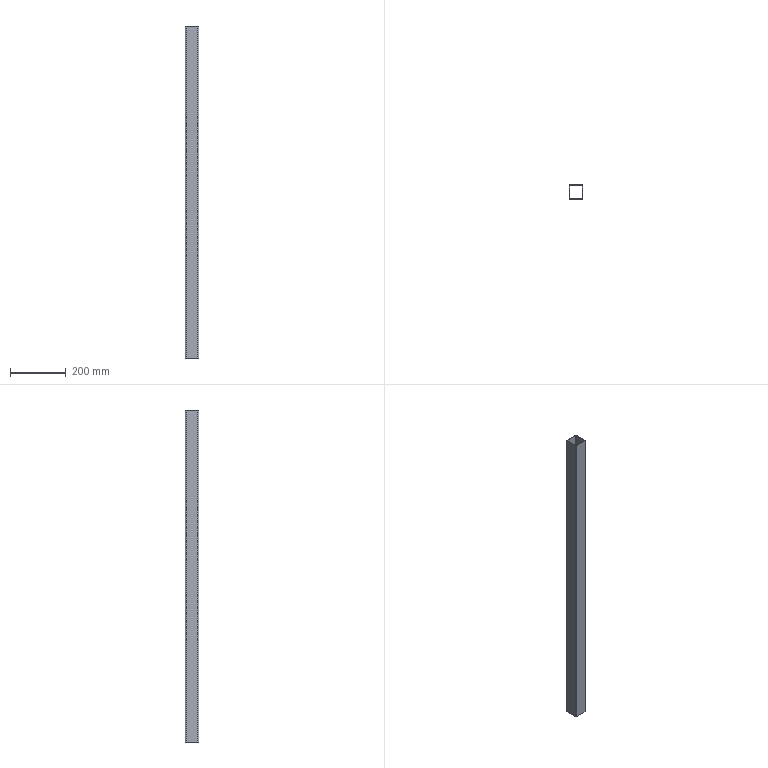Part | SolidWorks | features BaseBody 1 | 1 solid | 18 faces | box 50 x 50 x 1196 mm | volume 446944 mm3 | plane 10 | cylinder 8 | commonest cylinder face diameters 4 x4 8 x4
STEP:
#1=CARTESIAN_POINT('',(-23.,21.,-598.));
#2=VERTEX_POINT('',#1);
#3=CARTESIAN_POINT('',(-23.,-21.,-598.));
#4=VERTEX_POINT('',#3);
#5=CARTESIAN_POINT('',(-23.,21.,-598.));
#6=DIRECTION('',(0.,-1.,0.));
#7=VECTOR('',#6,1000.);
#8=LINE('',#5,#7);
#9=EDGE_CURVE('',#2,#4,#8,.T.);
#10=ORIENTED_EDGE('',*,*,#9,.F.);
#11=CARTESIAN_POINT('',(-23.,21.,598.));
#12=VERTEX_POINT('',#11);
#13=CARTESIAN_POINT('',(-23.,21.,598.));
#14=DIRECTION('',(0.,0.,-1.));
#15=VECTOR('',#14,1000.);
#16=LINE('',#13,#15);
#17=EDGE_CURVE('',#12,#2,#16,.T.);
#18=ORIENTED_EDGE('',*,*,#17,.F.);
#19=CARTESIAN_POINT('',(-23.,-21.,598.));
#20=VERTEX_POINT('',#19);
#21=CARTESIAN_POINT('',(-23.,21.,598.));
#22=DIRECTION('',(0.,-1.,0.));
#23=VECTOR('',#22,1000.);
#24=LINE('',#21,#23);
#25=EDGE_CURVE('',#12,#20,#24,.T.);
#26=ORIENTED_EDGE('',*,*,#25,.T.);
#27=CARTESIAN_POINT('',(-23.,-21.,598.));
#28=DIRECTION('',(0.,0.,-1.));
#29=VECTOR('',#28,1000.);
#30=LINE('',#27,#29);
#31=EDGE_CURVE('',#20,#4,#30,.T.);
#32=ORIENTED_EDGE('',*,*,#31,.T.);
#33=EDGE_LOOP('',(#10,#18,#26,#32));
#34=FACE_OUTER_BOUND('',#33,.T.);
#35=CARTESIAN_POINT('',(-23.,21.,598.));
#36=DIRECTION('',(1.,0.,0.));
#37=DIRECTION('',(0.,1.,0.));
#38=AXIS2_PLACEMENT_3D('',#35,#36,#37);
#39=PLANE('',#38);
#40=ADVANCED_FACE('',(#34),#39,.T.);
#41=CARTESIAN_POINT('',(-21.,23.,-598.));
#42=VERTEX_POINT('',#41);
#43=CARTESIAN_POINT('',(-21.,21.,-598.));
#44=DIRECTION('',(0.,0.,1.));
#45=DIRECTION('',(1.,0.,0.));
#46=AXIS2_PLACEMENT_3D('',#43,#44,#45);
#47=CIRCLE('',#46,2.);
#48=EDGE_CURVE('',#42,#2,#47,.T.);
#49=ORIENTED_EDGE('',*,*,#48,.F.);
#50=CARTESIAN_POINT('',(-21.,23.,598.));
#51=VERTEX_POINT('',#50);
#52=CARTESIAN_POINT('',(-21.,23.,598.));
#53=DIRECTION('',(0.,0.,-1.));
#54=VECTOR('',#53,1000.);
#55=LINE('',#52,#54);
#56=EDGE_CURVE('',#51,#42,#55,.T.);
#57=ORIENTED_EDGE('',*,*,#56,.F.);
#58=CARTESIAN_POINT('',(-21.,21.,598.));
#59=DIRECTION('',(0.,0.,1.));
#60=DIRECTION('',(1.,0.,0.));
#61=AXIS2_PLACEMENT_3D('',#58,#59,#60);
#62=CIRCLE('',#61,2.);
#63=EDGE_CURVE('',#51,#12,#62,.T.);
#64=ORIENTED_EDGE('',*,*,#63,.T.);
#65=ORIENTED_EDGE('',*,*,#17,.T.);
#66=EDGE_LOOP('',(#49,#57,#64,#65));
#67=FACE_OUTER_BOUND('',#66,.T.);
#68=CARTESIAN_POINT('',(-21.,21.,598.));
#69=DIRECTION('',(0.,0.,-1.));
#70=DIRECTION('',(-1.,0.,0.));
#71=AXIS2_PLACEMENT_3D('',#68,#69,#70);
#72=CYLINDRICAL_SURFACE('',#71,2.);
#73=ADVANCED_FACE('',(#67),#72,.F.);
#74=CARTESIAN_POINT('',(21.,23.,-598.));
#75=VERTEX_POINT('',#74);
#76=CARTESIAN_POINT('',(-21.,23.,-598.));
#77=DIRECTION('',(-1.,0.,0.));
#78=VECTOR('',#77,1000.);
#79=LINE('',#76,#78);
#80=EDGE_CURVE('',#75,#42,#79,.T.);
#81=ORIENTED_EDGE('',*,*,#80,.F.);
#82=CARTESIAN_POINT('',(21.,23.,598.));
#83=VERTEX_POINT('',#82);
#84=CARTESIAN_POINT('',(21.,23.,598.));
#85=DIRECTION('',(0.,0.,-1.));
#86=VECTOR('',#85,1000.);
#87=LINE('',#84,#86);
#88=EDGE_CURVE('',#83,#75,#87,.T.);
#89=ORIENTED_EDGE('',*,*,#88,.F.);
#90=CARTESIAN_POINT('',(-21.,23.,598.));
#91=DIRECTION('',(-1.,0.,0.));
#92=VECTOR('',#91,1000.);
#93=LINE('',#90,#92);
#94=EDGE_CURVE('',#83,#51,#93,.T.);
#95=ORIENTED_EDGE('',*,*,#94,.T.);
#96=ORIENTED_EDGE('',*,*,#56,.T.);
#97=EDGE_LOOP('',(#81,#89,#95,#96));
#98=FACE_OUTER_BOUND('',#97,.T.);
#99=CARTESIAN_POINT('',(-21.,23.,598.));
#100=DIRECTION('',(0.,-1.,0.));
#101=DIRECTION('',(0.,0.,-1.));
#102=AXIS2_PLACEMENT_3D('',#99,#100,#101);
#103=PLANE('',#102);
#104=ADVANCED_FACE('',(#98),#103,.T.);
#105=CARTESIAN_POINT('',(23.,21.,-598.));
#106=VERTEX_POINT('',#105);
#107=CARTESIAN_POINT('',(21.,21.,-598.));
#108=DIRECTION('',(0.,0.,1.));
#109=DIRECTION('',(1.,0.,0.));
#110=AXIS2_PLACEMENT_3D('',#107,#108,#109);
#111=CIRCLE('',#110,2.);
#112=EDGE_CURVE('',#106,#75,#111,.T.);
#113=ORIENTED_EDGE('',*,*,#112,.F.);
#114=CARTESIAN_POINT('',(23.,21.,598.));
#115=VERTEX_POINT('',#114);
#116=CARTESIAN_POINT('',(23.,21.,598.));
#117=DIRECTION('',(0.,0.,-1.));
#118=VECTOR('',#117,1000.);
#119=LINE('',#116,#118);
#120=EDGE_CURVE('',#115,#106,#119,.T.);
#121=ORIENTED_EDGE('',*,*,#120,.F.);
#122=CARTESIAN_POINT('',(21.,21.,598.));
#123=DIRECTION('',(0.,0.,1.));
#124=DIRECTION('',(1.,0.,0.));
#125=AXIS2_PLACEMENT_3D('',#122,#123,#124);
#126=CIRCLE('',#125,2.);
#127=EDGE_CURVE('',#115,#83,#126,.T.);
#128=ORIENTED_EDGE('',*,*,#127,.T.);
#129=ORIENTED_EDGE('',*,*,#88,.T.);
#130=EDGE_LOOP('',(#113,#121,#128,#129));
#131=FACE_OUTER_BOUND('',#130,.T.);
#132=CARTESIAN_POINT('',(21.,21.,598.));
#133=DIRECTION('',(0.,0.,-1.));
#134=DIRECTION('',(-1.,0.,0.));
#135=AXIS2_PLACEMENT_3D('',#132,#133,#134);
#136=CYLINDRICAL_SURFACE('',#135,2.);
#137=ADVANCED_FACE('',(#131),#136,.F.);
#138=CARTESIAN_POINT('',(23.,-21.,-598.));
#139=VERTEX_POINT('',#138);
#140=CARTESIAN_POINT('',(23.,21.,-598.));
#141=DIRECTION('',(0.,1.,0.));
#142=VECTOR('',#141,1000.);
#143=LINE('',#140,#142);
#144=EDGE_CURVE('',#139,#106,#143,.T.);
#145=ORIENTED_EDGE('',*,*,#144,.F.);
#146=CARTESIAN_POINT('',(23.,-21.,598.));
#147=VERTEX_POINT('',#146);
#148=CARTESIAN_POINT('',(23.,-21.,598.));
#149=DIRECTION('',(0.,0.,-1.));
#150=VECTOR('',#149,1000.);
#151=LINE('',#148,#150);
#152=EDGE_CURVE('',#147,#139,#151,.T.);
#153=ORIENTED_EDGE('',*,*,#152,.F.);
#154=CARTESIAN_POINT('',(23.,21.,598.));
#155=DIRECTION('',(0.,1.,0.));
#156=VECTOR('',#155,1000.);
#157=LINE('',#154,#156);
#158=EDGE_CURVE('',#147,#115,#157,.T.);
#159=ORIENTED_EDGE('',*,*,#158,.T.);
#160=ORIENTED_EDGE('',*,*,#120,.T.);
#161=EDGE_LOOP('',(#145,#153,#159,#160));
#162=FACE_OUTER_BOUND('',#161,.T.);
#163=CARTESIAN_POINT('',(23.,21.,598.));
#164=DIRECTION('',(-1.,0.,0.));
#165=DIRECTION('',(0.,1.,0.));
#166=AXIS2_PLACEMENT_3D('',#163,#164,#165);
#167=PLANE('',#166);
#168=ADVANCED_FACE('',(#162),#167,.T.);
#169=CARTESIAN_POINT('',(21.,-23.,-598.));
#170=VERTEX_POINT('',#169);
#171=CARTESIAN_POINT('',(21.,-21.,-598.));
#172=DIRECTION('',(0.,0.,1.));
#173=DIRECTION('',(1.,0.,0.));
#174=AXIS2_PLACEMENT_3D('',#171,#172,#173);
#175=CIRCLE('',#174,2.);
#176=EDGE_CURVE('',#170,#139,#175,.T.);
#177=ORIENTED_EDGE('',*,*,#176,.F.);
#178=CARTESIAN_POINT('',(21.,-23.,598.));
#179=VERTEX_POINT('',#178);
#180=CARTESIAN_POINT('',(21.,-23.,598.));
#181=DIRECTION('',(0.,0.,-1.));
#182=VECTOR('',#181,1000.);
#183=LINE('',#180,#182);
#184=EDGE_CURVE('',#179,#170,#183,.T.);
#185=ORIENTED_EDGE('',*,*,#184,.F.);
#186=CARTESIAN_POINT('',(21.,-21.,598.));
#187=DIRECTION('',(0.,0.,1.));
#188=DIRECTION('',(1.,0.,0.));
#189=AXIS2_PLACEMENT_3D('',#186,#187,#188);
#190=CIRCLE('',#189,2.);
#191=EDGE_CURVE('',#179,#147,#190,.T.);
#192=ORIENTED_EDGE('',*,*,#191,.T.);
#193=ORIENTED_EDGE('',*,*,#152,.T.);
#194=EDGE_LOOP('',(#177,#185,#192,#193));
#195=FACE_OUTER_BOUND('',#194,.T.);
#196=CARTESIAN_POINT('',(21.,-21.,598.));
#197=DIRECTION('',(0.,0.,-1.));
#198=DIRECTION('',(-1.,0.,0.));
#199=AXIS2_PLACEMENT_3D('',#196,#197,#198);
#200=CYLINDRICAL_SURFACE('',#199,2.);
#201=ADVANCED_FACE('',(#195),#200,.F.);
#202=CARTESIAN_POINT('',(-21.,-23.,-598.));
#203=VERTEX_POINT('',#202);
#204=CARTESIAN_POINT('',(-21.,-23.,-598.));
#205=DIRECTION('',(1.,0.,0.));
#206=VECTOR('',#205,1000.);
#207=LINE('',#204,#206);
#208=EDGE_CURVE('',#203,#170,#207,.T.);
#209=ORIENTED_EDGE('',*,*,#208,.F.);
#210=CARTESIAN_POINT('',(-21.,-23.,598.));
#211=VERTEX_POINT('',#210);
#212=CARTESIAN_POINT('',(-21.,-23.,598.));
#213=DIRECTION('',(0.,0.,-1.));
#214=VECTOR('',#213,1000.);
#215=LINE('',#212,#214);
#216=EDGE_CURVE('',#211,#203,#215,.T.);
#217=ORIENTED_EDGE('',*,*,#216,.F.);
#218=CARTESIAN_POINT('',(-21.,-23.,598.));
#219=DIRECTION('',(1.,0.,0.));
#220=VECTOR('',#219,1000.);
#221=LINE('',#218,#220);
#222=EDGE_CURVE('',#211,#179,#221,.T.);
#223=ORIENTED_EDGE('',*,*,#222,.T.);
#224=ORIENTED_EDGE('',*,*,#184,.T.);
#225=EDGE_LOOP('',(#209,#217,#223,#224));
#226=FACE_OUTER_BOUND('',#225,.T.);
#227=CARTESIAN_POINT('',(-21.,-23.,598.));
#228=DIRECTION('',(0.,1.,0.));
#229=DIRECTION('',(1.,0.,0.));
#230=AXIS2_PLACEMENT_3D('',#227,#228,#229);
#231=PLANE('',#230);
#232=ADVANCED_FACE('',(#226),#231,.T.);
#233=CARTESIAN_POINT('',(-21.,-21.,-598.));
#234=DIRECTION('',(0.,0.,1.));
#235=DIRECTION('',(1.,0.,0.));
#236=AXIS2_PLACEMENT_3D('',#233,#234,#235);
#237=CIRCLE('',#236,2.);
#238=EDGE_CURVE('',#4,#203,#237,.T.);
#239=ORIENTED_EDGE('',*,*,#238,.F.);
#240=ORIENTED_EDGE('',*,*,#31,.F.);
#241=CARTESIAN_POINT('',(-21.,-21.,598.));
#242=DIRECTION('',(0.,0.,1.));
#243=DIRECTION('',(1.,0.,0.));
#244=AXIS2_PLACEMENT_3D('',#241,#242,#243);
#245=CIRCLE('',#244,2.);
#246=EDGE_CURVE('',#20,#211,#245,.T.);
#247=ORIENTED_EDGE('',*,*,#246,.T.);
#248=ORIENTED_EDGE('',*,*,#216,.T.);
#249=EDGE_LOOP('',(#239,#240,#247,#248));
#250=FACE_OUTER_BOUND('',#249,.T.);
#251=CARTESIAN_POINT('',(-21.,-21.,598.));
#252=DIRECTION('',(0.,0.,-1.));
#253=DIRECTION('',(-1.,0.,0.));
#254=AXIS2_PLACEMENT_3D('',#251,#252,#253);
#255=CYLINDRICAL_SURFACE('',#254,2.);
#256=ADVANCED_FACE('',(#250),#255,.F.);
#257=CARTESIAN_POINT('',(-25.,21.,-598.));
#258=VERTEX_POINT('',#257);
#259=CARTESIAN_POINT('',(-25.,-21.,-598.));
#260=VERTEX_POINT('',#259);
#261=CARTESIAN_POINT('',(-25.,21.,-598.));
#262=DIRECTION('',(0.,-1.,0.));
#263=VECTOR('',#262,1000.);
#264=LINE('',#261,#263);
#265=EDGE_CURVE('',#258,#260,#264,.T.);
#266=ORIENTED_EDGE('',*,*,#265,.T.);
#267=CARTESIAN_POINT('',(-25.,-21.,598.));
#268=VERTEX_POINT('',#267);
#269=CARTESIAN_POINT('',(-25.,-21.,598.));
#270=DIRECTION('',(0.,0.,-1.));
#271=VECTOR('',#270,1000.);
#272=LINE('',#269,#271);
#273=EDGE_CURVE('',#268,#260,#272,.T.);
#274=ORIENTED_EDGE('',*,*,#273,.F.);
#275=CARTESIAN_POINT('',(-25.,21.,598.));
#276=VERTEX_POINT('',#275);
#277=CARTESIAN_POINT('',(-25.,21.,598.));
#278=DIRECTION('',(0.,-1.,0.));
#279=VECTOR('',#278,1000.);
#280=LINE('',#277,#279);
#281=EDGE_CURVE('',#276,#268,#280,.T.);
#282=ORIENTED_EDGE('',*,*,#281,.F.);
#283=CARTESIAN_POINT('',(-25.,21.,598.));
#284=DIRECTION('',(0.,0.,-1.));
#285=VECTOR('',#284,1000.);
#286=LINE('',#283,#285);
#287=EDGE_CURVE('',#276,#258,#286,.T.);
#288=ORIENTED_EDGE('',*,*,#287,.T.);
#289=EDGE_LOOP('',(#266,#274,#282,#288));
#290=FACE_OUTER_BOUND('',#289,.T.);
#291=CARTESIAN_POINT('',(-25.,21.,598.));
#292=DIRECTION('',(1.,0.,0.));
#293=DIRECTION('',(0.,1.,0.));
#294=AXIS2_PLACEMENT_3D('',#291,#292,#293);
#295=PLANE('',#294);
#296=ADVANCED_FACE('',(#290),#295,.F.);
#297=CARTESIAN_POINT('',(-21.,25.,-598.));
#298=VERTEX_POINT('',#297);
#299=CARTESIAN_POINT('',(-21.,21.,-598.));
#300=DIRECTION('',(0.,0.,1.));
#301=DIRECTION('',(1.,0.,0.));
#302=AXIS2_PLACEMENT_3D('',#299,#300,#301);
#303=CIRCLE('',#302,4.);
#304=EDGE_CURVE('',#298,#258,#303,.T.);
#305=ORIENTED_EDGE('',*,*,#304,.T.);
#306=ORIENTED_EDGE('',*,*,#287,.F.);
#307=CARTESIAN_POINT('',(-21.,25.,598.));
#308=VERTEX_POINT('',#307);
#309=CARTESIAN_POINT('',(-21.,21.,598.));
#310=DIRECTION('',(0.,0.,1.));
#311=DIRECTION('',(1.,0.,0.));
#312=AXIS2_PLACEMENT_3D('',#309,#310,#311);
#313=CIRCLE('',#312,4.);
#314=EDGE_CURVE('',#308,#276,#313,.T.);
#315=ORIENTED_EDGE('',*,*,#314,.F.);
#316=CARTESIAN_POINT('',(-21.,25.,598.));
#317=DIRECTION('',(0.,0.,-1.));
#318=VECTOR('',#317,1000.);
#319=LINE('',#316,#318);
#320=EDGE_CURVE('',#308,#298,#319,.T.);
#321=ORIENTED_EDGE('',*,*,#320,.T.);
#322=EDGE_LOOP('',(#305,#306,#315,#321));
#323=FACE_OUTER_BOUND('',#322,.T.);
#324=CARTESIAN_POINT('',(-21.,21.,598.));
#325=DIRECTION('',(0.,0.,-1.));
#326=DIRECTION('',(-1.,0.,0.));
#327=AXIS2_PLACEMENT_3D('',#324,#325,#326);
#328=CYLINDRICAL_SURFACE('',#327,4.);
#329=ADVANCED_FACE('',(#323),#328,.T.);
#330=CARTESIAN_POINT('',(21.,25.,-598.));
#331=VERTEX_POINT('',#330);
#332=CARTESIAN_POINT('',(-21.,25.,-598.));
#333=DIRECTION('',(-1.,0.,0.));
#334=VECTOR('',#333,1000.);
#335=LINE('',#332,#334);
#336=EDGE_CURVE('',#331,#298,#335,.T.);
#337=ORIENTED_EDGE('',*,*,#336,.T.);
#338=ORIENTED_EDGE('',*,*,#320,.F.);
#339=CARTESIAN_POINT('',(21.,25.,598.));
#340=VERTEX_POINT('',#339);
#341=CARTESIAN_POINT('',(-21.,25.,598.));
#342=DIRECTION('',(-1.,0.,0.));
#343=VECTOR('',#342,1000.);
#344=LINE('',#341,#343);
#345=EDGE_CURVE('',#340,#308,#344,.T.);
#346=ORIENTED_EDGE('',*,*,#345,.F.);
#347=CARTESIAN_POINT('',(21.,25.,598.));
#348=DIRECTION('',(0.,0.,-1.));
#349=VECTOR('',#348,1000.);
#350=LINE('',#347,#349);
#351=EDGE_CURVE('',#340,#331,#350,.T.);
#352=ORIENTED_EDGE('',*,*,#351,.T.);
#353=EDGE_LOOP('',(#337,#338,#346,#352));
#354=FACE_OUTER_BOUND('',#353,.T.);
#355=CARTESIAN_POINT('',(-21.,25.,598.));
#356=DIRECTION('',(0.,-1.,0.));
#357=DIRECTION('',(0.,0.,-1.));
#358=AXIS2_PLACEMENT_3D('',#355,#356,#357);
#359=PLANE('',#358);
#360=ADVANCED_FACE('',(#354),#359,.F.);
#361=CARTESIAN_POINT('',(25.,21.,-598.));
#362=VERTEX_POINT('',#361);
#363=CARTESIAN_POINT('',(21.,21.,-598.));
#364=DIRECTION('',(0.,0.,1.));
#365=DIRECTION('',(-1.,0.,0.));
#366=AXIS2_PLACEMENT_3D('',#363,#364,#365);
#367=CIRCLE('',#366,4.);
#368=EDGE_CURVE('',#362,#331,#367,.T.);
#369=ORIENTED_EDGE('',*,*,#368,.T.);
#370=ORIENTED_EDGE('',*,*,#351,.F.);
#371=CARTESIAN_POINT('',(25.,21.,598.));
#372=VERTEX_POINT('',#371);
#373=CARTESIAN_POINT('',(21.,21.,598.));
#374=DIRECTION('',(0.,0.,1.));
#375=DIRECTION('',(-1.,0.,0.));
#376=AXIS2_PLACEMENT_3D('',#373,#374,#375);
#377=CIRCLE('',#376,4.);
#378=EDGE_CURVE('',#372,#340,#377,.T.);
#379=ORIENTED_EDGE('',*,*,#378,.F.);
#380=CARTESIAN_POINT('',(25.,21.,598.));
#381=DIRECTION('',(0.,0.,-1.));
#382=VECTOR('',#381,1000.);
#383=LINE('',#380,#382);
#384=EDGE_CURVE('',#372,#362,#383,.T.);
#385=ORIENTED_EDGE('',*,*,#384,.T.);
#386=EDGE_LOOP('',(#369,#370,#379,#385));
#387=FACE_OUTER_BOUND('',#386,.T.);
#388=CARTESIAN_POINT('',(21.,21.,598.));
#389=DIRECTION('',(0.,0.,-1.));
#390=DIRECTION('',(-1.,0.,0.));
#391=AXIS2_PLACEMENT_3D('',#388,#389,#390);
#392=CYLINDRICAL_SURFACE('',#391,4.);
#393=ADVANCED_FACE('',(#387),#392,.T.);
#394=CARTESIAN_POINT('',(25.,-21.,-598.));
#395=VERTEX_POINT('',#394);
#396=CARTESIAN_POINT('',(25.,21.,-598.));
#397=DIRECTION('',(0.,1.,0.));
#398=VECTOR('',#397,1000.);
#399=LINE('',#396,#398);
#400=EDGE_CURVE('',#395,#362,#399,.T.);
#401=ORIENTED_EDGE('',*,*,#400,.T.);
#402=ORIENTED_EDGE('',*,*,#384,.F.);
#403=CARTESIAN_POINT('',(25.,-21.,598.));
#404=VERTEX_POINT('',#403);
#405=CARTESIAN_POINT('',(25.,21.,598.));
#406=DIRECTION('',(0.,1.,0.));
#407=VECTOR('',#406,1000.);
#408=LINE('',#405,#407);
#409=EDGE_CURVE('',#404,#372,#408,.T.);
#410=ORIENTED_EDGE('',*,*,#409,.F.);
#411=CARTESIAN_POINT('',(25.,-21.,598.));
#412=DIRECTION('',(0.,0.,-1.));
#413=VECTOR('',#412,1000.);
#414=LINE('',#411,#413);
#415=EDGE_CURVE('',#404,#395,#414,.T.);
#416=ORIENTED_EDGE('',*,*,#415,.T.);
#417=EDGE_LOOP('',(#401,#402,#410,#416));
#418=FACE_OUTER_BOUND('',#417,.T.);
#419=CARTESIAN_POINT('',(25.,21.,598.));
#420=DIRECTION('',(-1.,0.,0.));
#421=DIRECTION('',(0.,1.,0.));
#422=AXIS2_PLACEMENT_3D('',#419,#420,#421);
#423=PLANE('',#422);
#424=ADVANCED_FACE('',(#418),#423,.F.);
#425=CARTESIAN_POINT('',(21.,-25.,-598.));
#426=VERTEX_POINT('',#425);
#427=CARTESIAN_POINT('',(21.,-21.,-598.));
#428=DIRECTION('',(0.,0.,1.));
#429=DIRECTION('',(1.,0.,0.));
#430=AXIS2_PLACEMENT_3D('',#427,#428,#429);
#431=CIRCLE('',#430,4.);
#432=EDGE_CURVE('',#426,#395,#431,.T.);
#433=ORIENTED_EDGE('',*,*,#432,.T.);
#434=ORIENTED_EDGE('',*,*,#415,.F.);
#435=CARTESIAN_POINT('',(21.,-25.,598.));
#436=VERTEX_POINT('',#435);
#437=CARTESIAN_POINT('',(21.,-21.,598.));
#438=DIRECTION('',(0.,0.,1.));
#439=DIRECTION('',(1.,0.,0.));
#440=AXIS2_PLACEMENT_3D('',#437,#438,#439);
#441=CIRCLE('',#440,4.);
#442=EDGE_CURVE('',#436,#404,#441,.T.);
#443=ORIENTED_EDGE('',*,*,#442,.F.);
#444=CARTESIAN_POINT('',(21.,-25.,598.));
#445=DIRECTION('',(0.,0.,-1.));
#446=VECTOR('',#445,1000.);
#447=LINE('',#444,#446);
#448=EDGE_CURVE('',#436,#426,#447,.T.);
#449=ORIENTED_EDGE('',*,*,#448,.T.);
#450=EDGE_LOOP('',(#433,#434,#443,#449));
#451=FACE_OUTER_BOUND('',#450,.T.);
#452=CARTESIAN_POINT('',(21.,-21.,598.));
#453=DIRECTION('',(0.,0.,-1.));
#454=DIRECTION('',(-1.,0.,0.));
#455=AXIS2_PLACEMENT_3D('',#452,#453,#454);
#456=CYLINDRICAL_SURFACE('',#455,4.);
#457=ADVANCED_FACE('',(#451),#456,.T.);
#458=CARTESIAN_POINT('',(-21.,-25.,-598.));
#459=VERTEX_POINT('',#458);
#460=CARTESIAN_POINT('',(-21.,-25.,-598.));
#461=DIRECTION('',(1.,0.,0.));
#462=VECTOR('',#461,1000.);
#463=LINE('',#460,#462);
#464=EDGE_CURVE('',#459,#426,#463,.T.);
#465=ORIENTED_EDGE('',*,*,#464,.T.);
#466=ORIENTED_EDGE('',*,*,#448,.F.);
#467=CARTESIAN_POINT('',(-21.,-25.,598.));
#468=VERTEX_POINT('',#467);
#469=CARTESIAN_POINT('',(-21.,-25.,598.));
#470=DIRECTION('',(1.,0.,0.));
#471=VECTOR('',#470,1000.);
#472=LINE('',#469,#471);
#473=EDGE_CURVE('',#468,#436,#472,.T.);
#474=ORIENTED_EDGE('',*,*,#473,.F.);
#475=CARTESIAN_POINT('',(-21.,-25.,598.));
#476=DIRECTION('',(0.,0.,-1.));
#477=VECTOR('',#476,1000.);
#478=LINE('',#475,#477);
#479=EDGE_CURVE('',#468,#459,#478,.T.);
#480=ORIENTED_EDGE('',*,*,#479,.T.);
#481=EDGE_LOOP('',(#465,#466,#474,#480));
#482=FACE_OUTER_BOUND('',#481,.T.);
#483=CARTESIAN_POINT('',(-21.,-25.,598.));
#484=DIRECTION('',(0.,1.,0.));
#485=DIRECTION('',(1.,0.,0.));
#486=AXIS2_PLACEMENT_3D('',#483,#484,#485);
#487=PLANE('',#486);
#488=ADVANCED_FACE('',(#482),#487,.F.);
#489=CARTESIAN_POINT('',(-21.,-21.,-598.));
#490=DIRECTION('',(0.,0.,1.));
#491=DIRECTION('',(1.,0.,0.));
#492=AXIS2_PLACEMENT_3D('',#489,#490,#491);
#493=CIRCLE('',#492,4.);
#494=EDGE_CURVE('',#260,#459,#493,.T.);
#495=ORIENTED_EDGE('',*,*,#494,.T.);
#496=ORIENTED_EDGE('',*,*,#479,.F.);
#497=CARTESIAN_POINT('',(-21.,-21.,598.));
#498=DIRECTION('',(0.,0.,1.));
#499=DIRECTION('',(1.,0.,0.));
#500=AXIS2_PLACEMENT_3D('',#497,#498,#499);
#501=CIRCLE('',#500,4.);
#502=EDGE_CURVE('',#268,#468,#501,.T.);
#503=ORIENTED_EDGE('',*,*,#502,.F.);
#504=ORIENTED_EDGE('',*,*,#273,.T.);
#505=EDGE_LOOP('',(#495,#496,#503,#504));
#506=FACE_OUTER_BOUND('',#505,.T.);
#507=CARTESIAN_POINT('',(-21.,-21.,598.));
#508=DIRECTION('',(0.,0.,-1.));
#509=DIRECTION('',(-1.,0.,0.));
#510=AXIS2_PLACEMENT_3D('',#507,#508,#509);
#511=CYLINDRICAL_SURFACE('',#510,4.);
#512=ADVANCED_FACE('',(#506),#511,.T.);
#513=ORIENTED_EDGE('',*,*,#238,.T.);
#514=ORIENTED_EDGE('',*,*,#208,.T.);
#515=ORIENTED_EDGE('',*,*,#176,.T.);
#516=ORIENTED_EDGE('',*,*,#144,.T.);
#517=ORIENTED_EDGE('',*,*,#112,.T.);
#518=ORIENTED_EDGE('',*,*,#80,.T.);
#519=ORIENTED_EDGE('',*,*,#48,.T.);
#520=ORIENTED_EDGE('',*,*,#9,.T.);
#521=EDGE_LOOP('',(#513,#514,#515,#516,#517,#518,#519,#520));
#522=FACE_BOUND('',#521,.T.);
#523=ORIENTED_EDGE('',*,*,#494,.F.);
#524=ORIENTED_EDGE('',*,*,#265,.F.);
#525=ORIENTED_EDGE('',*,*,#304,.F.);
#526=ORIENTED_EDGE('',*,*,#336,.F.);
#527=ORIENTED_EDGE('',*,*,#368,.F.);
#528=ORIENTED_EDGE('',*,*,#400,.F.);
#529=ORIENTED_EDGE('',*,*,#432,.F.);
#530=ORIENTED_EDGE('',*,*,#464,.F.);
#531=EDGE_LOOP('',(#523,#524,#525,#526,#527,#528,#529,#530));
#532=FACE_OUTER_BOUND('',#531,.T.);
#533=CARTESIAN_POINT('',(-21.,-21.,-598.));
#534=DIRECTION('',(0.,0.,1.));
#535=DIRECTION('',(1.,0.,0.));
#536=AXIS2_PLACEMENT_3D('',#533,#534,#535);
#537=PLANE('',#536);
#538=ADVANCED_FACE('',(#522,#532),#537,.F.);
#539=ORIENTED_EDGE('',*,*,#222,.F.);
#540=ORIENTED_EDGE('',*,*,#246,.F.);
#541=ORIENTED_EDGE('',*,*,#25,.F.);
#542=ORIENTED_EDGE('',*,*,#63,.F.);
#543=ORIENTED_EDGE('',*,*,#94,.F.);
#544=ORIENTED_EDGE('',*,*,#127,.F.);
#545=ORIENTED_EDGE('',*,*,#158,.F.);
#546=ORIENTED_EDGE('',*,*,#191,.F.);
#547=EDGE_LOOP('',(#539,#540,#541,#542,#543,#544,#545,#546));
#548=FACE_BOUND('',#547,.T.);
#549=ORIENTED_EDGE('',*,*,#502,.T.);
#550=ORIENTED_EDGE('',*,*,#473,.T.);
#551=ORIENTED_EDGE('',*,*,#442,.T.);
#552=ORIENTED_EDGE('',*,*,#409,.T.);
#553=ORIENTED_EDGE('',*,*,#378,.T.);
#554=ORIENTED_EDGE('',*,*,#345,.T.);
#555=ORIENTED_EDGE('',*,*,#314,.T.);
#556=ORIENTED_EDGE('',*,*,#281,.T.);
#557=EDGE_LOOP('',(#549,#550,#551,#552,#553,#554,#555,#556));
#558=FACE_OUTER_BOUND('',#557,.T.);
#559=CARTESIAN_POINT('',(-21.,-21.,598.));
#560=DIRECTION('',(0.,0.,1.));
#561=DIRECTION('',(1.,0.,0.));
#562=AXIS2_PLACEMENT_3D('',#559,#560,#561);
#563=PLANE('',#562);
#564=ADVANCED_FACE('',(#548,#558),#563,.T.);
#565=CLOSED_SHELL('',(#40,#73,#104,#137,#168,#201,#232,#256,#296,#329,#360,#393,#424,#457,#488,#512,#538,#564));
#566=MANIFOLD_SOLID_BREP('',#565);
#567=CARTESIAN_POINT('',(0.,0.,0.));
#568=DIRECTION('',(0.,0.,1.));
#569=DIRECTION('',(1.,0.,0.));
#570=AXIS2_PLACEMENT_3D('',#567,#568,#569);
#571=(LENGTH_UNIT()NAMED_UNIT(*)SI_UNIT(.MILLI.,.METRE.));
#572=UNCERTAINTY_MEASURE_WITH_UNIT(LENGTH_MEASURE(0.00001),#571,'','');
#573=(NAMED_UNIT(*)PLANE_ANGLE_UNIT()SI_UNIT($,.RADIAN.));
#574=(NAMED_UNIT(*)SI_UNIT($,.STERADIAN.)SOLID_ANGLE_UNIT());
#575=(GEOMETRIC_REPRESENTATION_CONTEXT(3)GLOBAL_UNCERTAINTY_ASSIGNED_CONTEXT((#572))GLOBAL_UNIT_ASSIGNED_CONTEXT((#571,#573,#574))REPRESENTATION_CONTEXT('',''));
#576=ADVANCED_BREP_SHAPE_REPRESENTATION('',(#566,#570),#575);